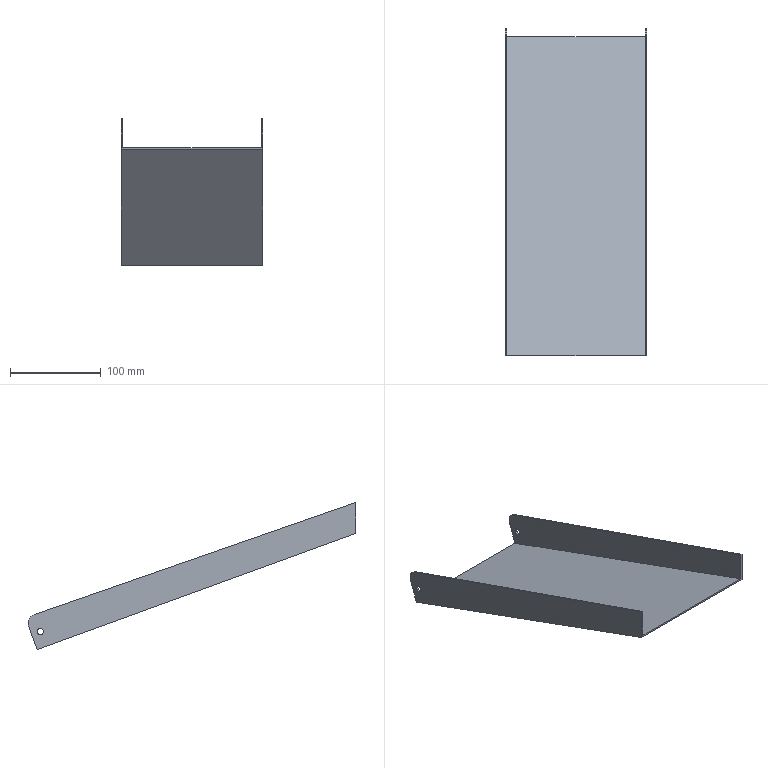Part | NX | features HB 2 | 1 solid | 14 faces | box 156 x 360.386 x 161.617 mm | volume 165851 mm3 | plane 10 | cylinder 4 | commonest cylinder face diameters 7 x2 20 x2
STEP:
#1=CARTESIAN_POINT('',(-38.,686.966,-375.785));
#2=VERTEX_POINT('',#1);
#3=CARTESIAN_POINT('',(-38.,686.966,-372.285));
#4=DIRECTION('',(1.,0.,0.));
#5=DIRECTION('',(0.,0.,-1.));
#6=AXIS2_PLACEMENT_3D('',#3,#4,#5);
#7=CIRCLE('',#6,3.5);
#8=EDGE_CURVE('',#2,#2,#7,.T.);
#9=ORIENTED_EDGE('',*,*,#8,.F.);
#10=EDGE_LOOP('',(#9));
#11=FACE_BOUND('',#10,.T.);
#12=CARTESIAN_POINT('',(-38.,691.161,-389.998));
#13=VERTEX_POINT('',#12);
#14=CARTESIAN_POINT('',(-38.,340.,-262.186));
#15=VERTEX_POINT('',#14);
#16=CARTESIAN_POINT('',(-38.,379.611,-276.603));
#17=DIRECTION('',(0.,-0.9397,0.342));
#18=VECTOR('',#17,1000.);
#19=LINE('',#16,#18);
#20=EDGE_CURVE('',#13,#15,#19,.T.);
#21=ORIENTED_EDGE('',*,*,#20,.F.);
#22=CARTESIAN_POINT('',(-38.,699.783,-366.309));
#23=VERTEX_POINT('',#22);
#24=CARTESIAN_POINT('',(-38.,692.943,-385.102));
#25=DIRECTION('',(0.,-0.342,-0.9397));
#26=VECTOR('',#25,1000.);
#27=LINE('',#24,#26);
#28=EDGE_CURVE('',#23,#13,#27,.T.);
#29=ORIENTED_EDGE('',*,*,#28,.F.);
#30=CARTESIAN_POINT('',(-38.,693.675,-353.445));
#31=VERTEX_POINT('',#30);
#32=CARTESIAN_POINT('',(-38.,690.386,-362.888));
#33=DIRECTION('',(-1.,0.,0.));
#34=DIRECTION('',(0.,0.,-1.));
#35=AXIS2_PLACEMENT_3D('',#32,#33,#34);
#36=CIRCLE('',#35,10.);
#37=EDGE_CURVE('',#31,#23,#36,.T.);
#38=ORIENTED_EDGE('',*,*,#37,.F.);
#39=CARTESIAN_POINT('',(-38.,340.,-230.26));
#40=VERTEX_POINT('',#39);
#41=CARTESIAN_POINT('',(-38.,390.115,-247.715));
#42=DIRECTION('',(0.,0.9444,-0.3289));
#43=VECTOR('',#42,1000.);
#44=LINE('',#41,#43);
#45=EDGE_CURVE('',#40,#31,#44,.T.);
#46=ORIENTED_EDGE('',*,*,#45,.F.);
#47=CARTESIAN_POINT('',(-38.,340.,-276.603));
#48=DIRECTION('',(0.,0.,1.));
#49=VECTOR('',#48,1000.);
#50=LINE('',#47,#49);
#51=EDGE_CURVE('',#15,#40,#50,.T.);
#52=ORIENTED_EDGE('',*,*,#51,.F.);
#53=EDGE_LOOP('',(#21,#29,#38,#46,#52));
#54=FACE_BOUND('',#53,.T.);
#55=CARTESIAN_POINT('',(-38.,379.611,-276.603));
#56=DIRECTION('',(1.,0.,0.));
#57=DIRECTION('',(0.,-0.08716,0.9962));
#58=AXIS2_PLACEMENT_3D('',#55,#56,#57);
#59=PLANE('',#58);
#60=ADVANCED_FACE('',(#11,#54),#59,.T.);
#61=CARTESIAN_POINT('',(114.,340.,-230.26));
#62=VERTEX_POINT('',#61);
#63=CARTESIAN_POINT('',(116.,340.,-230.26));
#64=VERTEX_POINT('',#63);
#65=CARTESIAN_POINT('',(-210.,340.,-230.26));
#66=DIRECTION('',(1.,0.,0.));
#67=VECTOR('',#66,1000.);
#68=LINE('',#65,#67);
#69=EDGE_CURVE('',#62,#64,#68,.T.);
#70=ORIENTED_EDGE('',*,*,#69,.T.);
#71=CARTESIAN_POINT('',(116.,693.675,-353.445));
#72=VERTEX_POINT('',#71);
#73=CARTESIAN_POINT('',(116.,390.115,-247.715));
#74=DIRECTION('',(0.,0.9444,-0.3289));
#75=VECTOR('',#74,1000.);
#76=LINE('',#73,#75);
#77=EDGE_CURVE('',#64,#72,#76,.T.);
#78=ORIENTED_EDGE('',*,*,#77,.T.);
#79=CARTESIAN_POINT('',(114.,693.675,-353.445));
#80=VERTEX_POINT('',#79);
#81=CARTESIAN_POINT('',(222.,693.675,-353.445));
#82=DIRECTION('',(1.,0.,0.));
#83=VECTOR('',#82,1000.);
#84=LINE('',#81,#83);
#85=EDGE_CURVE('',#80,#72,#84,.T.);
#86=ORIENTED_EDGE('',*,*,#85,.F.);
#87=CARTESIAN_POINT('',(114.,390.115,-247.715));
#88=DIRECTION('',(0.,0.9444,-0.3289));
#89=VECTOR('',#88,1000.);
#90=LINE('',#87,#89);
#91=EDGE_CURVE('',#62,#80,#90,.T.);
#92=ORIENTED_EDGE('',*,*,#91,.F.);
#93=EDGE_LOOP('',(#70,#78,#86,#92));
#94=FACE_BOUND('',#93,.T.);
#95=CARTESIAN_POINT('',(222.,390.115,-247.715));
#96=DIRECTION('',(0.,-0.3289,-0.9444));
#97=DIRECTION('',(0.,0.9444,-0.3289));
#98=AXIS2_PLACEMENT_3D('',#95,#96,#97);
#99=PLANE('',#98);
#100=ADVANCED_FACE('',(#94),#99,.F.);
#101=CARTESIAN_POINT('',(114.,686.661,-368.799));
#102=VERTEX_POINT('',#101);
#103=CARTESIAN_POINT('',(114.,686.966,-372.285));
#104=DIRECTION('',(-1.,0.,0.));
#105=DIRECTION('',(0.,-0.08716,0.9962));
#106=AXIS2_PLACEMENT_3D('',#103,#104,#105);
#107=CIRCLE('',#106,3.5);
#108=EDGE_CURVE('',#102,#102,#107,.T.);
#109=ORIENTED_EDGE('',*,*,#108,.F.);
#110=EDGE_LOOP('',(#109));
#111=FACE_BOUND('',#110,.T.);
#112=ORIENTED_EDGE('',*,*,#91,.T.);
#113=CARTESIAN_POINT('',(114.,699.783,-366.309));
#114=VERTEX_POINT('',#113);
#115=CARTESIAN_POINT('',(114.,690.386,-362.888));
#116=DIRECTION('',(1.,0.,0.));
#117=DIRECTION('',(0.,0.,1.));
#118=AXIS2_PLACEMENT_3D('',#115,#116,#117);
#119=CIRCLE('',#118,10.);
#120=EDGE_CURVE('',#114,#80,#119,.T.);
#121=ORIENTED_EDGE('',*,*,#120,.F.);
#122=CARTESIAN_POINT('',(114.,691.161,-389.998));
#123=VERTEX_POINT('',#122);
#124=CARTESIAN_POINT('',(114.,692.943,-385.102));
#125=DIRECTION('',(0.,-0.342,-0.9397));
#126=VECTOR('',#125,1000.);
#127=LINE('',#124,#126);
#128=EDGE_CURVE('',#114,#123,#127,.T.);
#129=ORIENTED_EDGE('',*,*,#128,.T.);
#130=CARTESIAN_POINT('',(114.,340.,-262.186));
#131=VERTEX_POINT('',#130);
#132=CARTESIAN_POINT('',(114.,379.611,-276.603));
#133=DIRECTION('',(0.,0.9397,-0.342));
#134=VECTOR('',#133,1000.);
#135=LINE('',#132,#134);
#136=EDGE_CURVE('',#131,#123,#135,.T.);
#137=ORIENTED_EDGE('',*,*,#136,.F.);
#138=CARTESIAN_POINT('',(114.,340.,-276.603));
#139=DIRECTION('',(0.,0.,-1.));
#140=VECTOR('',#139,1000.);
#141=LINE('',#138,#140);
#142=EDGE_CURVE('',#62,#131,#141,.T.);
#143=ORIENTED_EDGE('',*,*,#142,.F.);
#144=EDGE_LOOP('',(#112,#121,#129,#137,#143));
#145=FACE_BOUND('',#144,.T.);
#146=CARTESIAN_POINT('',(114.,379.611,-276.603));
#147=DIRECTION('',(-1.,0.,0.));
#148=DIRECTION('',(0.,-0.08716,0.9962));
#149=AXIS2_PLACEMENT_3D('',#146,#147,#148);
#150=PLANE('',#149);
#151=ADVANCED_FACE('',(#111,#145),#150,.T.);
#152=CARTESIAN_POINT('',(116.,686.661,-368.799));
#153=VERTEX_POINT('',#152);
#154=CARTESIAN_POINT('',(116.,686.966,-372.285));
#155=DIRECTION('',(-1.,0.,0.));
#156=DIRECTION('',(0.,-0.08716,0.9962));
#157=AXIS2_PLACEMENT_3D('',#154,#155,#156);
#158=CIRCLE('',#157,3.5);
#159=EDGE_CURVE('',#153,#153,#158,.T.);
#160=ORIENTED_EDGE('',*,*,#159,.T.);
#161=EDGE_LOOP('',(#160));
#162=FACE_BOUND('',#161,.T.);
#163=CARTESIAN_POINT('',(116.,340.,-264.314));
#164=VERTEX_POINT('',#163);
#165=CARTESIAN_POINT('',(116.,340.,-276.603));
#166=DIRECTION('',(0.,0.,-1.));
#167=VECTOR('',#166,1000.);
#168=LINE('',#165,#167);
#169=EDGE_CURVE('',#64,#164,#168,.T.);
#170=ORIENTED_EDGE('',*,*,#169,.T.);
#171=CARTESIAN_POINT('',(116.,690.477,-391.877));
#172=VERTEX_POINT('',#171);
#173=CARTESIAN_POINT('',(116.,378.927,-278.482));
#174=DIRECTION('',(0.,-0.9397,0.342));
#175=VECTOR('',#174,1000.);
#176=LINE('',#173,#175);
#177=EDGE_CURVE('',#172,#164,#176,.T.);
#178=ORIENTED_EDGE('',*,*,#177,.F.);
#179=CARTESIAN_POINT('',(116.,699.783,-366.309));
#180=VERTEX_POINT('',#179);
#181=CARTESIAN_POINT('',(116.,692.943,-385.102));
#182=DIRECTION('',(0.,-0.342,-0.9397));
#183=VECTOR('',#182,1000.);
#184=LINE('',#181,#183);
#185=EDGE_CURVE('',#180,#172,#184,.T.);
#186=ORIENTED_EDGE('',*,*,#185,.F.);
#187=CARTESIAN_POINT('',(116.,690.386,-362.888));
#188=DIRECTION('',(-1.,0.,0.));
#189=DIRECTION('',(0.,0.,1.));
#190=AXIS2_PLACEMENT_3D('',#187,#188,#189);
#191=CIRCLE('',#190,10.);
#192=EDGE_CURVE('',#72,#180,#191,.T.);
#193=ORIENTED_EDGE('',*,*,#192,.F.);
#194=ORIENTED_EDGE('',*,*,#77,.F.);
#195=EDGE_LOOP('',(#170,#178,#186,#193,#194));
#196=FACE_BOUND('',#195,.T.);
#197=CARTESIAN_POINT('',(116.,379.611,-276.603));
#198=DIRECTION('',(-1.,0.,0.));
#199=DIRECTION('',(0.,0.08716,-0.9962));
#200=AXIS2_PLACEMENT_3D('',#197,#198,#199);
#201=PLANE('',#200);
#202=ADVANCED_FACE('',(#162,#196),#201,.F.);
#203=CARTESIAN_POINT('',(-40.,340.,-264.314));
#204=VERTEX_POINT('',#203);
#205=CARTESIAN_POINT('',(-40.,690.477,-391.877));
#206=VERTEX_POINT('',#205);
#207=CARTESIAN_POINT('',(-40.,378.927,-278.482));
#208=DIRECTION('',(0.,0.9397,-0.342));
#209=VECTOR('',#208,1000.);
#210=LINE('',#207,#209);
#211=EDGE_CURVE('',#204,#206,#210,.T.);
#212=ORIENTED_EDGE('',*,*,#211,.T.);
#213=CARTESIAN_POINT('',(182.,690.477,-391.877));
#214=DIRECTION('',(1.,0.,0.));
#215=VECTOR('',#214,1000.);
#216=LINE('',#213,#215);
#217=EDGE_CURVE('',#206,#172,#216,.T.);
#218=ORIENTED_EDGE('',*,*,#217,.T.);
#219=ORIENTED_EDGE('',*,*,#177,.T.);
#220=CARTESIAN_POINT('',(182.,340.,-264.314));
#221=DIRECTION('',(-1.,0.,0.));
#222=VECTOR('',#221,1000.);
#223=LINE('',#220,#222);
#224=EDGE_CURVE('',#164,#204,#223,.T.);
#225=ORIENTED_EDGE('',*,*,#224,.T.);
#226=EDGE_LOOP('',(#212,#218,#219,#225));
#227=FACE_BOUND('',#226,.T.);
#228=CARTESIAN_POINT('',(182.,378.927,-278.482));
#229=DIRECTION('',(0.,0.342,0.9397));
#230=DIRECTION('',(-1.,0.,0.));
#231=AXIS2_PLACEMENT_3D('',#228,#229,#230);
#232=PLANE('',#231);
#233=ADVANCED_FACE('',(#227),#232,.F.);
#234=CARTESIAN_POINT('',(182.,340.,-262.186));
#235=DIRECTION('',(-1.,0.,0.));
#236=VECTOR('',#235,1000.);
#237=LINE('',#234,#236);
#238=EDGE_CURVE('',#131,#15,#237,.T.);
#239=ORIENTED_EDGE('',*,*,#238,.F.);
#240=ORIENTED_EDGE('',*,*,#136,.T.);
#241=CARTESIAN_POINT('',(182.,691.161,-389.998));
#242=DIRECTION('',(1.,0.,0.));
#243=VECTOR('',#242,1000.);
#244=LINE('',#241,#243);
#245=EDGE_CURVE('',#13,#123,#244,.T.);
#246=ORIENTED_EDGE('',*,*,#245,.F.);
#247=ORIENTED_EDGE('',*,*,#20,.T.);
#248=EDGE_LOOP('',(#239,#240,#246,#247));
#249=FACE_BOUND('',#248,.T.);
#250=CARTESIAN_POINT('',(182.,379.611,-276.603));
#251=DIRECTION('',(0.,0.342,0.9397));
#252=DIRECTION('',(-1.,0.,0.));
#253=AXIS2_PLACEMENT_3D('',#250,#251,#252);
#254=PLANE('',#253);
#255=ADVANCED_FACE('',(#249),#254,.T.);
#256=CARTESIAN_POINT('',(-40.,340.,-230.26));
#257=VERTEX_POINT('',#256);
#258=CARTESIAN_POINT('',(-208.,340.,-230.26));
#259=DIRECTION('',(1.,0.,0.));
#260=VECTOR('',#259,1000.);
#261=LINE('',#258,#260);
#262=EDGE_CURVE('',#257,#40,#261,.T.);
#263=ORIENTED_EDGE('',*,*,#262,.T.);
#264=ORIENTED_EDGE('',*,*,#45,.T.);
#265=CARTESIAN_POINT('',(-40.,693.675,-353.445));
#266=VERTEX_POINT('',#265);
#267=CARTESIAN_POINT('',(184.,693.675,-353.445));
#268=DIRECTION('',(1.,0.,0.));
#269=VECTOR('',#268,1000.);
#270=LINE('',#267,#269);
#271=EDGE_CURVE('',#266,#31,#270,.T.);
#272=ORIENTED_EDGE('',*,*,#271,.F.);
#273=CARTESIAN_POINT('',(-40.,390.115,-247.715));
#274=DIRECTION('',(0.,0.9444,-0.3289));
#275=VECTOR('',#274,1000.);
#276=LINE('',#273,#275);
#277=EDGE_CURVE('',#257,#266,#276,.T.);
#278=ORIENTED_EDGE('',*,*,#277,.F.);
#279=EDGE_LOOP('',(#263,#264,#272,#278));
#280=FACE_BOUND('',#279,.T.);
#281=CARTESIAN_POINT('',(-48.,390.115,-247.715));
#282=DIRECTION('',(0.,-0.3289,-0.9444));
#283=DIRECTION('',(0.,0.9444,-0.3289));
#284=AXIS2_PLACEMENT_3D('',#281,#282,#283);
#285=PLANE('',#284);
#286=ADVANCED_FACE('',(#280),#285,.F.);
#287=CARTESIAN_POINT('',(-40.,686.966,-375.785));
#288=VERTEX_POINT('',#287);
#289=CARTESIAN_POINT('',(-40.,686.966,-372.285));
#290=DIRECTION('',(-1.,0.,0.));
#291=DIRECTION('',(0.,0.,-1.));
#292=AXIS2_PLACEMENT_3D('',#289,#290,#291);
#293=CIRCLE('',#292,3.5);
#294=EDGE_CURVE('',#288,#288,#293,.T.);
#295=ORIENTED_EDGE('',*,*,#294,.F.);
#296=EDGE_LOOP('',(#295));
#297=FACE_BOUND('',#296,.T.);
#298=CARTESIAN_POINT('',(-40.,340.,-276.603));
#299=DIRECTION('',(0.,0.,1.));
#300=VECTOR('',#299,1000.);
#301=LINE('',#298,#300);
#302=EDGE_CURVE('',#204,#257,#301,.T.);
#303=ORIENTED_EDGE('',*,*,#302,.T.);
#304=ORIENTED_EDGE('',*,*,#277,.T.);
#305=CARTESIAN_POINT('',(-40.,699.783,-366.309));
#306=VERTEX_POINT('',#305);
#307=CARTESIAN_POINT('',(-40.,690.386,-362.888));
#308=DIRECTION('',(1.,0.,0.));
#309=DIRECTION('',(0.,0.,-1.));
#310=AXIS2_PLACEMENT_3D('',#307,#308,#309);
#311=CIRCLE('',#310,10.);
#312=EDGE_CURVE('',#306,#266,#311,.T.);
#313=ORIENTED_EDGE('',*,*,#312,.F.);
#314=CARTESIAN_POINT('',(-40.,692.943,-385.102));
#315=DIRECTION('',(0.,-0.342,-0.9397));
#316=VECTOR('',#315,1000.);
#317=LINE('',#314,#316);
#318=EDGE_CURVE('',#306,#206,#317,.T.);
#319=ORIENTED_EDGE('',*,*,#318,.T.);
#320=ORIENTED_EDGE('',*,*,#211,.F.);
#321=EDGE_LOOP('',(#303,#304,#313,#319,#320));
#322=FACE_BOUND('',#321,.T.);
#323=CARTESIAN_POINT('',(-40.,379.611,-276.603));
#324=DIRECTION('',(1.,0.,0.));
#325=DIRECTION('',(0.,-0.08716,0.9962));
#326=AXIS2_PLACEMENT_3D('',#323,#324,#325);
#327=PLANE('',#326);
#328=ADVANCED_FACE('',(#297,#322),#327,.F.);
#329=ORIENTED_EDGE('',*,*,#108,.T.);
#330=EDGE_LOOP('',(#329));
#331=FACE_BOUND('',#330,.T.);
#332=ORIENTED_EDGE('',*,*,#159,.F.);
#333=EDGE_LOOP('',(#332));
#334=FACE_BOUND('',#333,.T.);
#335=CARTESIAN_POINT('',(826.,686.966,-372.285));
#336=DIRECTION('',(-1.,0.,0.));
#337=DIRECTION('',(0.,0.08716,-0.9962));
#338=AXIS2_PLACEMENT_3D('',#335,#336,#337);
#339=CYLINDRICAL_SURFACE('',#338,3.5);
#340=ADVANCED_FACE('',(#331,#334),#339,.F.);
#341=ORIENTED_EDGE('',*,*,#120,.T.);
#342=ORIENTED_EDGE('',*,*,#85,.T.);
#343=ORIENTED_EDGE('',*,*,#192,.T.);
#344=CARTESIAN_POINT('',(222.,699.783,-366.309));
#345=DIRECTION('',(-1.,0.,0.));
#346=VECTOR('',#345,1000.);
#347=LINE('',#344,#346);
#348=EDGE_CURVE('',#180,#114,#347,.T.);
#349=ORIENTED_EDGE('',*,*,#348,.T.);
#350=EDGE_LOOP('',(#341,#342,#343,#349));
#351=FACE_BOUND('',#350,.T.);
#352=CARTESIAN_POINT('',(222.,690.386,-362.888));
#353=DIRECTION('',(-1.,0.,0.));
#354=DIRECTION('',(0.,0.,-1.));
#355=AXIS2_PLACEMENT_3D('',#352,#353,#354);
#356=CYLINDRICAL_SURFACE('',#355,10.);
#357=ADVANCED_FACE('',(#351),#356,.T.);
#358=ORIENTED_EDGE('',*,*,#245,.T.);
#359=ORIENTED_EDGE('',*,*,#128,.F.);
#360=ORIENTED_EDGE('',*,*,#348,.F.);
#361=ORIENTED_EDGE('',*,*,#185,.T.);
#362=ORIENTED_EDGE('',*,*,#217,.F.);
#363=ORIENTED_EDGE('',*,*,#318,.F.);
#364=CARTESIAN_POINT('',(184.,699.783,-366.309));
#365=DIRECTION('',(-1.,0.,0.));
#366=VECTOR('',#365,1000.);
#367=LINE('',#364,#366);
#368=EDGE_CURVE('',#23,#306,#367,.T.);
#369=ORIENTED_EDGE('',*,*,#368,.F.);
#370=ORIENTED_EDGE('',*,*,#28,.T.);
#371=EDGE_LOOP('',(#358,#359,#360,#361,#362,#363,#369,#370));
#372=FACE_BOUND('',#371,.T.);
#373=CARTESIAN_POINT('',(182.,692.943,-385.102));
#374=DIRECTION('',(0.,-0.9397,0.342));
#375=DIRECTION('',(0.,-0.342,-0.9397));
#376=AXIS2_PLACEMENT_3D('',#373,#374,#375);
#377=PLANE('',#376);
#378=ADVANCED_FACE('',(#372),#377,.F.);
#379=ORIENTED_EDGE('',*,*,#37,.T.);
#380=ORIENTED_EDGE('',*,*,#368,.T.);
#381=ORIENTED_EDGE('',*,*,#312,.T.);
#382=ORIENTED_EDGE('',*,*,#271,.T.);
#383=EDGE_LOOP('',(#379,#380,#381,#382));
#384=FACE_BOUND('',#383,.T.);
#385=CARTESIAN_POINT('',(184.,690.386,-362.888));
#386=DIRECTION('',(1.,0.,0.));
#387=DIRECTION('',(0.,0.,1.));
#388=AXIS2_PLACEMENT_3D('',#385,#386,#387);
#389=CYLINDRICAL_SURFACE('',#388,10.);
#390=ADVANCED_FACE('',(#384),#389,.T.);
#391=ORIENTED_EDGE('',*,*,#8,.T.);
#392=EDGE_LOOP('',(#391));
#393=FACE_BOUND('',#392,.T.);
#394=ORIENTED_EDGE('',*,*,#294,.T.);
#395=EDGE_LOOP('',(#394));
#396=FACE_BOUND('',#395,.T.);
#397=CARTESIAN_POINT('',(857.,686.966,-372.285));
#398=DIRECTION('',(-1.,0.,0.));
#399=DIRECTION('',(0.,0.08716,-0.9962));
#400=AXIS2_PLACEMENT_3D('',#397,#398,#399);
#401=CYLINDRICAL_SURFACE('',#400,3.5);
#402=ADVANCED_FACE('',(#393,#396),#401,.F.);
#403=ORIENTED_EDGE('',*,*,#69,.F.);
#404=ORIENTED_EDGE('',*,*,#142,.T.);
#405=ORIENTED_EDGE('',*,*,#238,.T.);
#406=ORIENTED_EDGE('',*,*,#51,.T.);
#407=ORIENTED_EDGE('',*,*,#262,.F.);
#408=ORIENTED_EDGE('',*,*,#302,.F.);
#409=ORIENTED_EDGE('',*,*,#224,.F.);
#410=ORIENTED_EDGE('',*,*,#169,.F.);
#411=EDGE_LOOP('',(#403,#404,#405,#406,#407,#408,#409,#410));
#412=FACE_BOUND('',#411,.T.);
#413=CARTESIAN_POINT('',(-210.,340.,60.));
#414=DIRECTION('',(0.,-1.,0.));
#415=DIRECTION('',(0.,0.,-1.));
#416=AXIS2_PLACEMENT_3D('',#413,#414,#415);
#417=PLANE('',#416);
#418=ADVANCED_FACE('',(#412),#417,.T.);
#419=CLOSED_SHELL('',(#60,#100,#151,#202,#233,#255,#286,#328,#340,#357,#378,#390,#402,#418));
#420=MANIFOLD_SOLID_BREP('',#419);
#421=(LENGTH_UNIT()NAMED_UNIT(*)SI_UNIT(.MILLI.,.METRE.));
#422=UNCERTAINTY_MEASURE_WITH_UNIT(LENGTH_MEASURE(0.00001),#421,'','');
#423=(NAMED_UNIT(*)PLANE_ANGLE_UNIT()SI_UNIT($,.RADIAN.));
#424=(NAMED_UNIT(*)SI_UNIT($,.STERADIAN.)SOLID_ANGLE_UNIT());
#425=(GEOMETRIC_REPRESENTATION_CONTEXT(3)GLOBAL_UNCERTAINTY_ASSIGNED_CONTEXT((#422))GLOBAL_UNIT_ASSIGNED_CONTEXT((#421,#423,#424))REPRESENTATION_CONTEXT('',''));
#426=ADVANCED_BREP_SHAPE_REPRESENTATION('',(#420),#425);